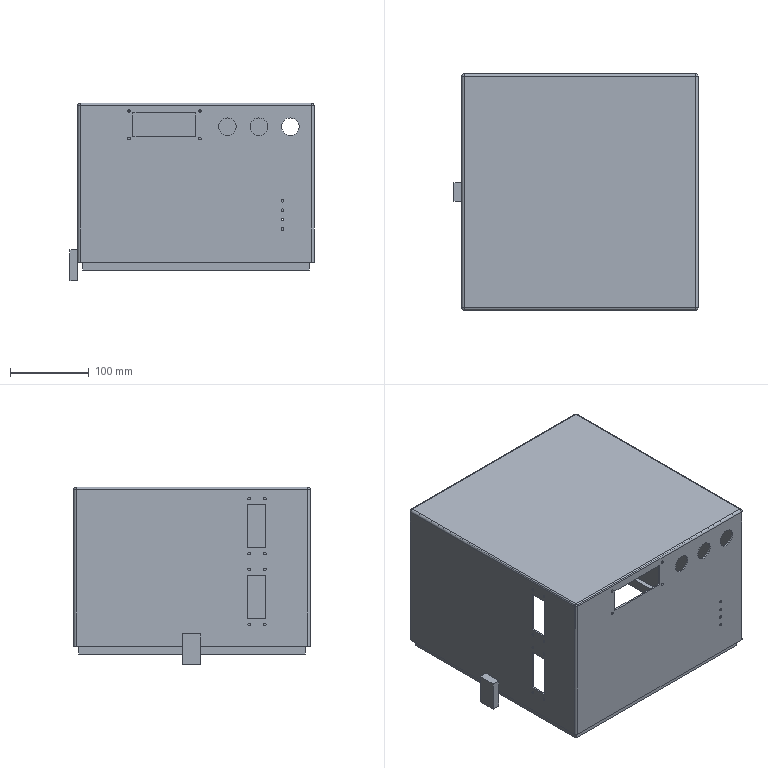Part | STEP file | Station two ctrl box body | 1 solid | 171 faces | box 310 x 300 x 225.796 mm | volume 688947 mm3 | cylinder 86 | plane 81 | spline 4 | commonest cylinder face diameters 3.3 x40 5 x12 22.5 x12 6 x8 9 x6 6.5 x4